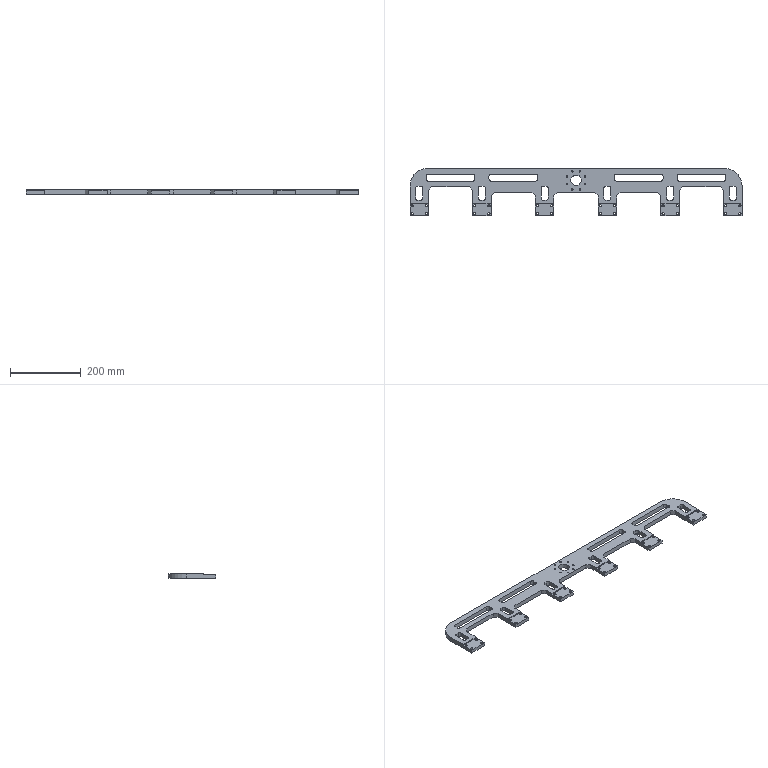NC program | NX | posted with a generic post | part box 941 x 134 x 13 mm
Lines 8393 to 8798 of 8798:
(PLANAR_MILL_COPY_1 , TOOL : D6A45)
N16724 T07 M6
N16726 G54
N16728 G17 G0 G90 X-452.4 Y-2.13 S9500 M3
N16730 G43 Z30. H7
N16732 Z0.
N16734 G94 G1 Z-1. F1400.
N16736 X-453.1 Y-2.534
N16738 G3 X-453.6 Y-3.4 R1.
N16740 G1 Y-17.4
N16742 G3 X-448.5 Y-22.5 R5.1
N16744 G1 X-440.5
N16746 G3 X-435.4 Y-17.4 R5.1
N16748 G1 Y10.6
N16750 G3 X-440.5 Y15.7 R5.1
N16752 G1 X-448.5
N16754 G3 X-453.6 Y10.6 R5.1
N16756 G1 Y-3.4
N16758 G3 X-453.1 Y-4.266 R1.
N16760 G1 X-452.4 Y-4.67
N16762 Z0.
N16764 G0 Z30.
N16766 X-354.33 Y48.9
N16768 Z0.
N16770 G1 Z-1.
N16772 X-354.734 Y49.6
N16774 G3 X-355.6 Y50.1 R1.
N16776 G1 X-418.5
N16778 G3 X-423.6 Y45. R5.1
N16780 G1 Y37.
N16782 G3 X-418.5 Y31.9 R5.1
N16784 G1 X-292.7
N16786 G3 X-287.6 Y37. R5.1
N16788 G1 Y45.
N16790 G3 X-292.7 Y50.1 R5.1
N16792 G1 X-355.6
N16794 G3 X-356.466 Y49.6 R1.
N16796 G1 X-356.87 Y48.9
N16798 Z0.
N16800 G0 Z30.
N16802 X-274.6 Y-2.13
N16804 Z0.
N16806 G1 Z-1.
N16808 X-275.3 Y-2.534
N16810 G3 X-275.8 Y-3.4 R1.
N16812 G1 Y-17.4
N16814 G3 X-270.7 Y-22.5 R5.1
N16816 G1 X-262.7
N16818 G3 X-257.6 Y-17.4 R5.1
N16820 G1 Y10.6
N16822 G3 X-262.7 Y15.7 R5.1
N16824 G1 X-270.7
N16826 G3 X-275.8 Y10.6 R5.1
N16828 G1 Y-3.4
N16830 G3 X-275.3 Y-4.266 R1.
N16832 G1 X-274.6 Y-4.67
N16834 Z0.
N16836 G0 Z30.
N16838 X-176.53 Y48.9
N16840 Z0.
N16842 G1 Z-1.
N16844 X-176.934 Y49.6
N16846 G3 X-177.8 Y50.1 R1.
N16848 G1 X-240.7
N16850 G3 X-245.8 Y45. R5.1
N16852 G1 Y37.
N16854 G3 X-240.7 Y31.9 R5.1
N16856 G1 X-114.9
N16858 G3 X-109.8 Y37. R5.1
N16860 G1 Y45.
N16862 G3 X-114.9 Y50.1 R5.1
N16864 G1 X-177.8
N16866 G3 X-178.666 Y49.6 R1.
N16868 G1 X-179.07 Y48.9
N16870 Z0.
N16872 G0 Z30.
N16874 X-96.8 Y-2.13
N16876 Z0.
N16878 G1 Z-1.
N16880 X-97.5 Y-2.534
N16882 G3 X-98. Y-3.4 R1.
N16884 G1 Y-17.4
N16886 G3 X-92.9 Y-22.5 R5.1
N16888 G1 X-84.9
N16890 G3 X-79.8 Y-17.4 R5.1
N16892 G1 Y10.6
N16894 G3 X-84.9 Y15.7 R5.1
N16896 G1 X-92.9
N16898 G3 X-98. Y10.6 R5.1
N16900 G1 Y-3.4
N16902 G3 X-97.5 Y-4.266 R1.
N16904 G1 X-96.8 Y-4.67
N16906 Z0.
N16908 G0 Z30.
N16910 X-25.662 Y22.39
N16912 Z0.
N16914 G1 Z-1.
N16916 X-24.903 Y23.135
N16918 G3 X-25.769 Y23.635 R1.
N16920 X-27.119 Y22.285 R1.35
N16922 X-25.769 Y23.635 R-1.35
N16924 X-26.635 Y23.135 R1.
N16926 G1 X-25.876 Y22.39
N16928 Z0.
N16930 G0 Z30.
N16932 X-10.722 Y7.026
N16934 Z0.
N16936 G1 Z-1.
N16938 X-11.481 Y6.281
N16940 G3 X-10.615 Y5.781 R1.
N16942 X-9.265 Y7.131 R1.35
N16944 X-10.615 Y5.781 R-1.35
N16946 X-9.749 Y6.281 R1.
N16948 G1 X-10.508 Y7.026
N16950 Z0.
N16952 G0 Z30.
N16954 X10.708
N16956 Z0.
N16958 G1 Z-1.
N16960 X9.949 Y6.281
N16962 G3 X10.815 Y5.781 R1.
N16964 X12.165 Y7.131 R1.35
N16966 X10.815 Y5.781 R-1.35
N16968 X11.681 Y6.281 R1.
N16970 G1 X10.922 Y7.026
N16972 Z0.
N16974 G0 Z30.
N16976 X1.409 Y45.833
N16978 Z0.
N16980 G1 Z-1.
N16982 X0.966 Y46.6
N16984 G3 X0.1 Y47.1 R1.
N16986 X-14. Y33. R14.1
N16988 X0.1 Y47.1 R-14.1
N16990 X-0.766 Y46.6 R1.
N16992 G1 X-1.209 Y45.833
N16994 Z0.
N16996 G0 Z30.
N16998 X-25.662 Y43.82
N17000 Z0.
N17002 G1 Z-1.
N17004 X-24.903 Y44.565
N17006 G3 X-25.769 Y45.065 R1.
N17008 X-27.119 Y43.715 R1.35
N17010 X-25.769 Y45.065 R-1.35
N17012 X-26.635 Y44.565 R1.
N17014 G1 X-25.876 Y43.82
N17016 Z0.
N17018 G0 Z30.
N17020 X-10.508 Y58.974
N17022 Z0.
N17024 G1 Z-1.
N17026 X-9.749 Y59.719
N17028 G3 X-10.615 Y60.219 R1.
N17030 X-11.965 Y58.869 R1.35
N17032 X-10.615 Y60.219 R-1.35
N17034 X-11.481 Y59.719 R1.
N17036 G1 X-10.722 Y58.974
N17038 Z0.
N17040 G0 Z30.
N17042 X10.922
N17044 Z0.
N17046 G1 Z-1.
N17048 X11.681 Y59.719
N17050 G3 X10.815 Y60.219 R1.
N17052 X9.465 Y58.869 R1.35
N17054 X10.815 Y60.219 R-1.35
N17056 X9.949 Y59.719 R1.
N17058 G1 X10.708 Y58.974
N17060 Z0.
N17062 G0 Z30.
N17064 X26.076 Y43.82
N17066 Z0.
N17068 G1 Z-1.
N17070 X26.835 Y44.565
N17072 G3 X25.969 Y45.065 R1.
N17074 X24.619 Y43.715 R1.35
N17076 X25.969 Y45.065 R-1.35
N17078 X25.103 Y44.565 R1.
N17080 G1 X25.862 Y43.82
N17082 Z0.
N17084 G0 Z30.
N17086 X26.076 Y22.39
N17088 Z0.
N17090 G1 Z-1.
N17092 X26.835 Y23.135
N17094 G3 X25.969 Y23.635 R1.
N17096 X24.619 Y22.285 R1.35
N17098 X25.969 Y23.635 R-1.35
N17100 X25.103 Y23.135 R1.
N17102 G1 X25.862 Y22.39
N17104 Z0.
N17106 G0 Z30.
N17108 X64.359 Y-35.5
N17110 Z0.
N17112 G1 Z-1.
N17114 X63.955 Y-34.8
N17116 G3 X63.089 Y-34.3 R1.
N17118 G1 X63.
N17120 G2 X62. Y-33.3 R1.
N17122 G1 Y-11.328
N17124 X52.527 Y-1.855
N17126 X-52.527
N17128 X-62. Y-11.328
N17130 Y-33.3
N17132 G2 X-63. Y-34.3 R1.
N17134 G1 X-114.8
N17136 G2 X-115.8 Y-33.3 R1.
N17138 G1 Y-11.328
N17140 X-125.273 Y-1.855
N17142 X-230.327
N17144 X-239.8 Y-11.328
N17146 Y-33.3
N17148 G2 X-240.8 Y-34.3 R1.
N17150 G1 X-292.6
N17152 G2 X-293.6 Y-33.3 R1.
N17154 G1 Y4.627
N17156 X-303.073 Y14.1
N17158 X-408.127
N17160 X-417.6 Y4.627
N17162 Y-33.3
N17164 G2 X-418.6 Y-34.3 R1.
N17166 G1 X-470.4
N17168 G2 X-471.4 Y-33.3 R1.
N17170 G1 Y17.
N17172 G2 X-420.5 Y67.9 R50.9
N17174 G1 X63.089
N17176 G3 X63.955 Y68.4 R1.
N17178 G1 X64.359 Y69.1
N17180 Z0.
N17182 G0 Z30.
(PLANAR_MILL_COPY_COPY , TOOL : D6A45)
N17184 X-60.587 Y-37.492
N17186 Z-3.
N17188 G1 Z-4.
N17190 X-61.035 Y-37.043
N17192 G3 X-62. Y-36.782 R1.
N17194 G1 Y-66.9
N17196 G2 X-63. Y-67.9 R1.
N17198 G1 X-114.8
N17200 G2 X-115.8 Y-66.9 R1.
N17202 G1 Y-36.782
N17204 G3 X-116.765 Y-37.043 R1.
N17206 G1 X-117.213 Y-37.492
N17208 Z-3.
N17210 G0 Z30.
N17212 X-238.387
N17214 Z-3.
N17216 G1 Z-4.
N17218 X-238.835 Y-37.043
N17220 G3 X-239.8 Y-36.782 R1.
N17222 G1 Y-66.9
N17224 G2 X-240.8 Y-67.9 R1.
N17226 G1 X-292.6
N17228 G2 X-293.6 Y-66.9 R1.
N17230 G1 Y-36.782
N17232 G3 X-294.565 Y-37.043 R1.
N17234 G1 X-295.013 Y-37.492
N17236 Z-3.
N17238 G0 Z30.
N17240 X-416.187
N17242 Z-3.
N17244 G1 Z-4.
N17246 X-416.635 Y-37.043
N17248 G3 X-417.6 Y-36.782 R1.
N17250 G1 Y-66.9
N17252 G2 X-418.6 Y-67.9 R1.
N17254 G1 X-470.4
N17256 G2 X-471.4 Y-66.9 R1.
N17258 G1 Y-36.782
N17260 G3 X-472.365 Y-37.043 R1.
N17262 G1 X-472.813 Y-37.492
N17264 Z-3.
N17266 G0 Z30.
N17268 X-69.388 Y-62.242
N17270 Z-3.
N17272 G1 Z-4.
N17274 X-69.766 Y-63.05
N17276 G3 X-68.9 Y-63.55 R1.
N17278 X-66.55 Y-61.2 R2.35
N17280 X-68.9 Y-63.55 R-2.35
N17282 X-68.034 Y-63.05 R1.
N17284 G1 X-68.412 Y-62.242
N17286 Z-3.
N17288 G0 Z30.
N17290 X-68.907 Y-38.1
N17292 Z-3.
N17294 G1 Z-4.
N17296 Y-37.056
N17298 G3 X-69.382 Y-36.9 R0.5
N17300 X-68.418 Y-36.9 R-2.35
N17302 X-68.893 Y-37.056 R0.5
N17304 G1 Y-38.1
N17306 Z-3.
N17308 G0 Z30.
N17310 X-108.907
N17312 Z-3.
N17314 G1 Z-4.
N17316 Y-37.056
N17318 G3 X-109.382 Y-36.9 R0.5
N17320 X-108.418 Y-36.9 R-2.35
N17322 X-108.893 Y-37.056 R0.5
N17324 G1 Y-38.1
N17326 Z-3.
N17328 G0 Z30.
N17330 X-109.388 Y-62.242
N17332 Z-3.
N17334 G1 Z-4.
N17336 X-109.766 Y-63.05
N17338 G3 X-108.9 Y-63.55 R1.
N17340 X-106.55 Y-61.2 R2.35
N17342 X-108.9 Y-63.55 R-2.35
N17344 X-108.034 Y-63.05 R1.
N17346 G1 X-108.412 Y-62.242
N17348 Z-3.
N17350 G0 Z30.
N17352 X-247.188
N17354 Z-3.
N17356 G1 Z-4.
N17358 X-247.566 Y-63.05
N17360 G3 X-246.7 Y-63.55 R1.
N17362 X-244.35 Y-61.2 R2.35
N17364 X-246.7 Y-63.55 R-2.35
N17366 X-245.834 Y-63.05 R1.
N17368 G1 X-246.212 Y-62.242
N17370 Z-3.
N17372 G0 Z30.
N17374 X-246.707 Y-38.1
N17376 Z-3.
N17378 G1 Z-4.
N17380 Y-37.056
N17382 G3 X-247.182 Y-36.9 R0.5
N17384 X-246.218 Y-36.9 R-2.35
N17386 X-246.693 Y-37.056 R0.5
N17388 G1 Y-38.1
N17390 Z-3.
N17392 G0 Z30.
N17394 X-286.707
N17396 Z-3.
N17398 G1 Z-4.
N17400 Y-37.056
N17402 G3 X-287.182 Y-36.9 R0.5
N17404 X-286.218 Y-36.9 R-2.35
N17406 X-286.693 Y-37.056 R0.5
N17408 G1 Y-38.1
N17410 Z-3.
N17412 G0 Z30.
N17414 X-287.188 Y-62.242
N17416 Z-3.
N17418 G1 Z-4.
N17420 X-287.566 Y-63.05
N17422 G3 X-286.7 Y-63.55 R1.
N17424 X-284.35 Y-61.2 R2.35
N17426 X-286.7 Y-63.55 R-2.35
N17428 X-285.834 Y-63.05 R1.
N17430 G1 X-286.212 Y-62.242
N17432 Z-3.
N17434 G0 Z30.
N17436 X-424.988
N17438 Z-3.
N17440 G1 Z-4.
N17442 X-425.366 Y-63.05
N17444 G3 X-424.5 Y-63.55 R1.
N17446 X-422.15 Y-61.2 R2.35
N17448 X-424.5 Y-63.55 R-2.35
N17450 X-423.634 Y-63.05 R1.
N17452 G1 X-424.012 Y-62.242
N17454 Z-3.
N17456 G0 Z30.
N17458 X-424.507 Y-38.1
N17460 Z-3.
N17462 G1 Z-4.
N17464 Y-37.056
N17466 G3 X-424.982 Y-36.9 R0.5
N17468 X-424.018 Y-36.9 R-2.35
N17470 X-424.493 Y-37.056 R0.5
N17472 G1 Y-38.1
N17474 Z-3.
N17476 G0 Z30.
N17478 X-464.507
N17480 Z-3.
N17482 G1 Z-4.
N17484 Y-37.056
N17486 G3 X-464.982 Y-36.9 R0.5
N17488 X-464.018 Y-36.9 R-2.35
N17490 X-464.493 Y-37.056 R0.5
N17492 G1 Y-38.1
N17494 Z-3.
N17496 G0 Z30.
N17498 X-464.988 Y-62.242
N17500 Z-3.
N17502 G1 Z-4.
N17504 X-465.366 Y-63.05
N17506 G3 X-464.5 Y-63.55 R1.
N17508 X-462.15 Y-61.2 R2.35
N17510 X-464.5 Y-63.55 R-2.35
N17512 X-463.634 Y-63.05 R1.
N17514 G1 X-464.012 Y-62.242
N17516 Z-3.
N17518 G0 Z30.
N17520 M5
N17522 M2